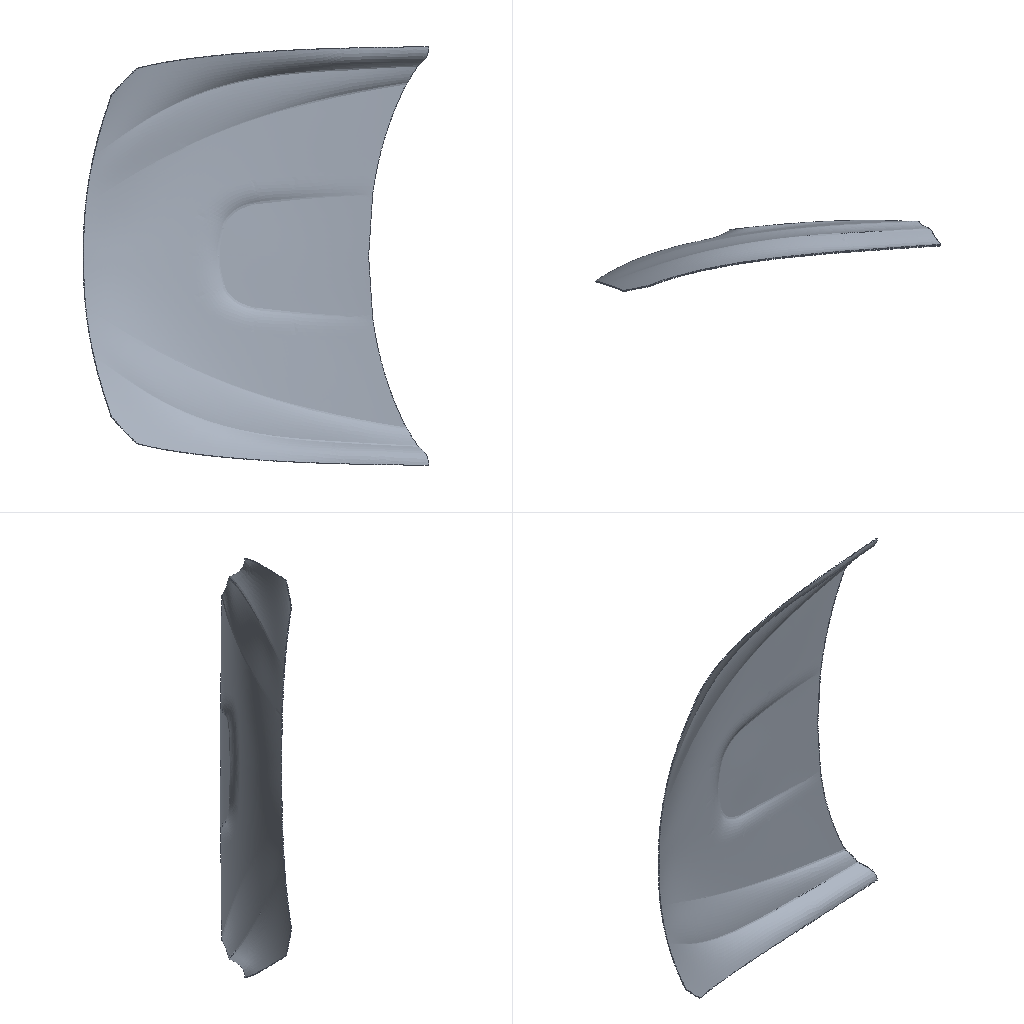Simulation study | nx simcenter
Set-up summary:
category,name,step,type,value,unit,region
solver,nx_nastran (Simcenter)
units,not stated in the deck,,not stated
analysis,deck,,static,static
analysis,solution,,SOL,101
load_step,SUBCASE 1,1,SUBCASE,SPC=1 LOAD=2
load_step,requested,,,1
mesh,nodes,,,139261
mesh,elements,,,68817
element_type,CTETRA,,solid,68817
load,nodal force total,,FX,0.0,model units
load,nodal force total,,FY,0.0,model units
load,nodal force total,,FZ,0.0,model units
load,load commands in deck,,count,17942
bc,support commands in deck,,count,41974
analysis,NX solution 0,,Structural,SESTATIC 101 - Single Constraint
analysis,NX solution 0,,Structural,SESTATIC 101 - Single Constraint
check,setup vs results,,match,every grid point's frame and coordinates and every element id; grid points of CTETRA elements
Nastran input file, long lists of numbers shortened:
$*$$$$$$$$$$$$$$$$$$$$$$$$$$$$$$$$$$$$$$$$$$$$$$$$$$$$$$$$$$$$$$$$$
$*
$*                    Simcenter v12.0.0.27 Translator
$*                    for NX Nastran version 12.0
$ (40 more lines like these left out)
ID,NASTRAN,盖子_fem2_sim1-solution_1
SOL 101
CEND
$*
$*$$$$$$$$$$$$$$$$$$$$$$$$$$$$$$$$$$$
$*
$* CASE CONTROL
$*
$*$$$$$$$$$$$$$$$$$$$$$$$$$$$$$$$$$$$
$*
ECHO = NONE
SPC = 1
OUTPUT
DISPLACEMENT(PLOT,REAL) = ALL
SPCFORCES(PLOT,REAL) = ALL
STRESS(PLOT,REAL,VONMISES,CENTER) = ALL
$*  Step: Subcase - Static Loads 1
SUBCASE 1
  LABEL = Subcase - Static Loads 1
  LOAD = 2
$*
$*$$$$$$$$$$$$$$$$$$$$$$$$$$$$$$$$$$$
$*
$* BULK DATA
$*
$*$$$$$$$$$$$$$$$$$$$$$$$$$$$$$$$$$$$
$*
BEGIN BULK
$*
$* PARAM CARDS
$*
PARAM      K6ROT100.0000
PARAM     OIBULK     YES
PARAM    OMACHPR     YES
PARAM       POST      -2
PARAM    POSTEXT     YES
PARAM    UNITSYS   MN-MM
$*
$* GRID CARDS
$*
GRID*                  1               0-3.475979117E+037.5668800684E+02+
*       -2.224163306E+02               0
GRID*                  2               0-3.484124529E+037.3121540616E+02+
*       3.7367580306E+02               0
$ (278518 more lines like these left out)
$*
$* ELEMENT CARDS
$*
$*  Mesh Collector: Solid(2)
$*  Mesh: 3d_mesh(1)
CTETRA         1       2   60356   95162   95180   95181      18   95408+
+             19      20   95407   95410
CTETRA         2       2  131620  138852  131454   60362  131622      21+
+             22   60561   60562      23
$ (137630 more lines like these left out)
$*
$* PROPERTY CARDS
$*
$*  Property: PSOLID2
PSOLID         2       1       0                           SMECH
$*
$* MATERIAL CARDS
$*
$*  Material: AISI_410_SS::盖子_fem2::[1]
MAT1           12.1936+8        0.2680007.7338-69.6800-6
MATT1          1       1               2               3
TABLEM1        1                       1                                +
+        20.00002.1936+8 21.11002.1936+8 23.89002.1936+8 37.78002.1867+8+
+        51.67002.1729+8 65.56002.1660+8 79.44002.1591+8 93.33002.1453+8+
+       107.22002.1384+8121.11002.1315+8135.00002.1177+8148.89002.1108+8+
+       162.78002.1039+8176.67002.0901+8190.56002.0832+8204.44002.0694+8+
+       218.33002.0625+8232.22002.0556+8246.11002.0418+8260.00002.0349+8+
+       273.89002.0211+8287.78002.0142+8301.67002.0004+8315.56001.9935+8+
+       329.44001.9866+8343.33001.9728+8357.22001.9659+8371.11001.9521+8+
+       385.00001.9452+8398.89001.9314+8412.78001.9176+8426.67001.9038+8+
+       440.56001.8900+8454.44001.8763+8468.33001.8625+8482.22001.8418+8+
+       496.11001.8280+8510.00001.8073+8523.89001.7866+8537.78001.7659+8+
+       551.67001.7452+8565.56001.7176+8579.44001.6969+8593.33001.6693+8+
+       607.22001.6417+8621.11001.6141+8635.00001.5796+8648.89001.5520+8+
+       662.78001.5176+8676.67001.4831+8690.56001.4417+8704.44001.4072+8+
+           ENDT
TABLEM1        2                       1                                +
+        20.00000.268000 21.11000.268000 23.89000.268000 37.78000.268000+
+        51.67000.268000 65.56000.268000 79.44000.268000 93.33000.268000+
+       107.22000.268000121.11000.268000135.00000.268000148.89000.268000+
+       162.78000.268000176.67000.268000190.56000.268000204.44000.268000+
+       218.33000.268000232.22000.268000246.11000.268000260.00000.268000+
+       273.89000.268000287.78000.268000301.67000.268000315.56000.268000+
+       329.44000.269000343.33000.269000357.22000.269000371.11000.269000+
+       385.00000.270000398.89000.270000412.78000.271000426.67000.271000+
+       440.56000.272000454.44000.273000468.33000.274000482.22000.275000+
+       496.11000.277000510.00000.278000523.89000.280000537.78000.281000+
+       551.67000.283000565.56000.286000579.44000.288000593.33000.290000+
+       607.22000.293000621.11000.295000635.00000.298000648.89000.301000+
+       662.78000.305000676.67000.308000690.56000.311000704.44000.315000+
+           ENDT
TABLEM1        3                       1                                +
+        20.00009.6800-6 93.33001.0080-5107.22001.0152-5121.11001.0224-5+
+       135.00001.0296-5148.89001.0368-5162.78001.0440-5176.67001.0512-5+
+       190.56001.0566-5204.44001.0638-5218.33001.0710-5232.22001.0764-5+
+       246.11001.0836-5260.00001.0890-5273.89001.0944-5287.78001.1016-5+
+       301.67001.1070-5315.56001.1124-5329.44001.1178-5343.33001.1232-5+
+       357.22001.1286-5371.11001.1340-5385.00001.1394-5398.89001.1448-5+
+       412.78001.1484-5426.67001.1538-5440.56001.1574-5454.44001.1610-5+
+       468.33001.1646-5482.22001.1682-5496.11001.1718-5510.00001.1754-5+
+       523.89001.1790-5537.78001.1826-5551.67001.1862-5565.56001.1880-5+
+       579.44001.1916-5593.33001.1952-5607.22001.1988-5621.11001.2006-5+
+       635.00001.2042-5648.89001.2060-5662.78001.2096-5676.67001.2114-5+
+       690.56001.2150-5704.44001.2186-5718.33001.2222-5732.22001.2258-5+
+       746.11001.2294-5760.00001.2348-5773.89001.2384-5787.78001.2438-5+
+       801.67001.2474-5815.56001.2528-5829.44001.2582-5843.33001.2654-5+
+       857.22001.2726-5871.11001.2798-5885.00001.2888-5898.89001.2978-5+
+       912.78001.3068-5926.67001.3158-5940.56001.3266-5954.44001.3374-5+
+       968.33001.3464-5982.22001.3572-5996.11001.3680-5 1010.001.3806-5+
+        1023.891.3914-5 1037.781.4022-5    ENDT
$*
$* LOAD AND CONSTRAINT CARDS
$*
$*  Constraint: Fixed(1)
SPC            1   48275  123456  0.0000
SPC            1   48276  123456  0.0000
SPC            1   48277  123456  0.0000
SPC            1   48278  123456  0.0000
$ (41970 more lines like these left out)
$*  Load: Pressure(1)
PLOAD4         2       5 5000.00                          117942   88670
PLOAD4         2      21 5000.00                          130916  130898
PLOAD4         2      29 5000.00                           69621  137430
PLOAD4         2      36 5000.00                           54267  138688
$ (17938 more lines like these left out)
ENDDATA 087f4876
Results summary:
result,analysis,,,static
result,last_loadstep,,,1
result,primary field,,,displacements
result,max displacement,,,0.000304,model units
result,reaction total,,FX,-1724528640.0,model units
result,reaction total,,FY,7661668352.0,model units
result,reaction total,,FZ,-168511424.0,model units
result,NX solution 0,,loadcases,1,mm
result,NX solution 0,,loadcases